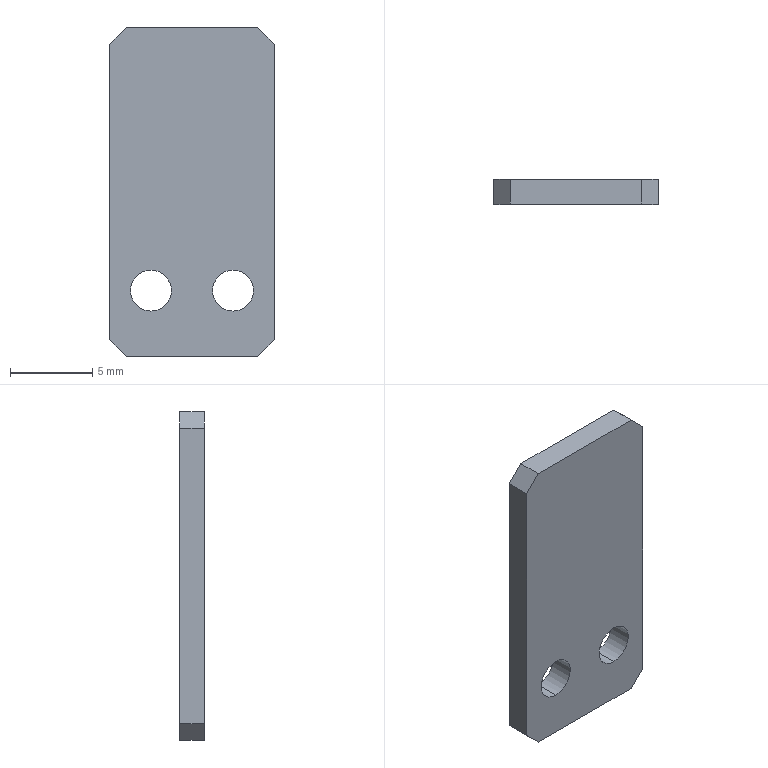Part | SolidWorks | features 3DProfileFeature 1, Chamfer 1, Extrusion 1, HoleWzd 1 | 1 solid | 14 faces | box 10 x 1.5 x 20 mm | volume 282.274 mm3 | plane 10 | cylinder 4 | commonest cylinder face diameters 2.5 x4
STEP:
#1=CARTESIAN_POINT('',(-2.5,0.,-7.25));
#2=VERTEX_POINT('',#1);
#3=CARTESIAN_POINT('',(-2.5,0.,-4.75));
#4=VERTEX_POINT('',#3);
#5=CARTESIAN_POINT('',(-2.5,0.,-6.));
#6=DIRECTION('',(0.,1.,0.));
#7=DIRECTION('',(0.,0.,1.));
#8=AXIS2_PLACEMENT_3D('',#5,#6,#7);
#9=CIRCLE('',#8,1.25);
#10=EDGE_CURVE('',#2,#4,#9,.T.);
#11=ORIENTED_EDGE('',*,*,#10,.F.);
#12=CARTESIAN_POINT('',(-2.5,1.5,-7.25));
#13=VERTEX_POINT('',#12);
#14=CARTESIAN_POINT('',(-2.5,1.5,-7.25));
#15=DIRECTION('',(0.,1.,0.));
#16=VECTOR('',#15,1000.);
#17=LINE('',#14,#16);
#18=EDGE_CURVE('',#2,#13,#17,.T.);
#19=ORIENTED_EDGE('',*,*,#18,.T.);
#20=CARTESIAN_POINT('',(-2.5,1.5,-4.75));
#21=VERTEX_POINT('',#20);
#22=CARTESIAN_POINT('',(-2.5,1.5,-6.));
#23=DIRECTION('',(0.,1.,0.));
#24=DIRECTION('',(0.,0.,1.));
#25=AXIS2_PLACEMENT_3D('',#22,#23,#24);
#26=CIRCLE('',#25,1.25);
#27=EDGE_CURVE('',#13,#21,#26,.T.);
#28=ORIENTED_EDGE('',*,*,#27,.T.);
#29=CARTESIAN_POINT('',(-2.5,1.5,-4.75));
#30=DIRECTION('',(0.,1.,0.));
#31=VECTOR('',#30,1000.);
#32=LINE('',#29,#31);
#33=EDGE_CURVE('',#4,#21,#32,.T.);
#34=ORIENTED_EDGE('',*,*,#33,.F.);
#35=EDGE_LOOP('',(#11,#19,#28,#34));
#36=FACE_OUTER_BOUND('',#35,.T.);
#37=CARTESIAN_POINT('',(-2.5,1.5,-6.));
#38=DIRECTION('',(0.,1.,0.));
#39=DIRECTION('',(0.,0.,1.));
#40=AXIS2_PLACEMENT_3D('',#37,#38,#39);
#41=CYLINDRICAL_SURFACE('',#40,1.25);
#42=ADVANCED_FACE('',(#36),#41,.F.);
#43=CARTESIAN_POINT('',(2.5,0.,-7.25));
#44=VERTEX_POINT('',#43);
#45=CARTESIAN_POINT('',(2.5,0.,-4.75));
#46=VERTEX_POINT('',#45);
#47=CARTESIAN_POINT('',(2.5,0.,-6.));
#48=DIRECTION('',(0.,1.,0.));
#49=DIRECTION('',(0.,0.,1.));
#50=AXIS2_PLACEMENT_3D('',#47,#48,#49);
#51=CIRCLE('',#50,1.25);
#52=EDGE_CURVE('',#44,#46,#51,.T.);
#53=ORIENTED_EDGE('',*,*,#52,.F.);
#54=CARTESIAN_POINT('',(2.5,1.5,-7.25));
#55=VERTEX_POINT('',#54);
#56=CARTESIAN_POINT('',(2.5,1.5,-7.25));
#57=DIRECTION('',(0.,1.,0.));
#58=VECTOR('',#57,1000.);
#59=LINE('',#56,#58);
#60=EDGE_CURVE('',#44,#55,#59,.T.);
#61=ORIENTED_EDGE('',*,*,#60,.T.);
#62=CARTESIAN_POINT('',(2.5,1.5,-4.75));
#63=VERTEX_POINT('',#62);
#64=CARTESIAN_POINT('',(2.5,1.5,-6.));
#65=DIRECTION('',(0.,1.,0.));
#66=DIRECTION('',(0.,0.,1.));
#67=AXIS2_PLACEMENT_3D('',#64,#65,#66);
#68=CIRCLE('',#67,1.25);
#69=EDGE_CURVE('',#55,#63,#68,.T.);
#70=ORIENTED_EDGE('',*,*,#69,.T.);
#71=CARTESIAN_POINT('',(2.5,1.5,-4.75));
#72=DIRECTION('',(0.,1.,0.));
#73=VECTOR('',#72,1000.);
#74=LINE('',#71,#73);
#75=EDGE_CURVE('',#46,#63,#74,.T.);
#76=ORIENTED_EDGE('',*,*,#75,.F.);
#77=EDGE_LOOP('',(#53,#61,#70,#76));
#78=FACE_OUTER_BOUND('',#77,.T.);
#79=CARTESIAN_POINT('',(2.5,1.5,-6.));
#80=DIRECTION('',(0.,1.,0.));
#81=DIRECTION('',(0.,0.,1.));
#82=AXIS2_PLACEMENT_3D('',#79,#80,#81);
#83=CYLINDRICAL_SURFACE('',#82,1.25);
#84=ADVANCED_FACE('',(#78),#83,.F.);
#85=CARTESIAN_POINT('',(5.,1.5,9.));
#86=VERTEX_POINT('',#85);
#87=CARTESIAN_POINT('',(5.,1.5,-9.));
#88=VERTEX_POINT('',#87);
#89=CARTESIAN_POINT('',(5.,1.5,-10.));
#90=DIRECTION('',(0.,0.,-1.));
#91=VECTOR('',#90,1000.);
#92=LINE('',#89,#91);
#93=EDGE_CURVE('',#86,#88,#92,.T.);
#94=ORIENTED_EDGE('',*,*,#93,.F.);
#95=CARTESIAN_POINT('',(5.,0.,9.));
#96=VERTEX_POINT('',#95);
#97=CARTESIAN_POINT('',(5.,1.5,9.));
#98=DIRECTION('',(0.,-1.,0.));
#99=VECTOR('',#98,1000.);
#100=LINE('',#97,#99);
#101=EDGE_CURVE('',#86,#96,#100,.T.);
#102=ORIENTED_EDGE('',*,*,#101,.T.);
#103=CARTESIAN_POINT('',(5.,0.,-9.));
#104=VERTEX_POINT('',#103);
#105=CARTESIAN_POINT('',(5.,0.,-10.));
#106=DIRECTION('',(0.,0.,-1.));
#107=VECTOR('',#106,1000.);
#108=LINE('',#105,#107);
#109=EDGE_CURVE('',#96,#104,#108,.T.);
#110=ORIENTED_EDGE('',*,*,#109,.T.);
#111=CARTESIAN_POINT('',(5.,1.5,-9.));
#112=DIRECTION('',(0.,1.,0.));
#113=VECTOR('',#112,1000.);
#114=LINE('',#111,#113);
#115=EDGE_CURVE('',#104,#88,#114,.T.);
#116=ORIENTED_EDGE('',*,*,#115,.T.);
#117=EDGE_LOOP('',(#94,#102,#110,#116));
#118=FACE_OUTER_BOUND('',#117,.T.);
#119=CARTESIAN_POINT('',(5.,1.5,-10.));
#120=DIRECTION('',(-1.,0.,0.));
#121=DIRECTION('',(0.,0.,1.));
#122=AXIS2_PLACEMENT_3D('',#119,#120,#121);
#123=PLANE('',#122);
#124=ADVANCED_FACE('',(#118),#123,.F.);
#125=CARTESIAN_POINT('',(4.,1.5,-10.));
#126=VERTEX_POINT('',#125);
#127=CARTESIAN_POINT('',(-4.,1.5,-10.));
#128=VERTEX_POINT('',#127);
#129=CARTESIAN_POINT('',(-5.,1.5,-10.));
#130=DIRECTION('',(-1.,0.,0.));
#131=VECTOR('',#130,1000.);
#132=LINE('',#129,#131);
#133=EDGE_CURVE('',#126,#128,#132,.T.);
#134=ORIENTED_EDGE('',*,*,#133,.F.);
#135=CARTESIAN_POINT('',(4.,0.,-10.));
#136=VERTEX_POINT('',#135);
#137=CARTESIAN_POINT('',(4.,1.5,-10.));
#138=DIRECTION('',(0.,-1.,0.));
#139=VECTOR('',#138,1000.);
#140=LINE('',#137,#139);
#141=EDGE_CURVE('',#126,#136,#140,.T.);
#142=ORIENTED_EDGE('',*,*,#141,.T.);
#143=CARTESIAN_POINT('',(-4.,0.,-10.));
#144=VERTEX_POINT('',#143);
#145=CARTESIAN_POINT('',(-5.,0.,-10.));
#146=DIRECTION('',(-1.,0.,0.));
#147=VECTOR('',#146,1000.);
#148=LINE('',#145,#147);
#149=EDGE_CURVE('',#136,#144,#148,.T.);
#150=ORIENTED_EDGE('',*,*,#149,.T.);
#151=CARTESIAN_POINT('',(-4.,1.5,-10.));
#152=DIRECTION('',(0.,1.,0.));
#153=VECTOR('',#152,1000.);
#154=LINE('',#151,#153);
#155=EDGE_CURVE('',#144,#128,#154,.T.);
#156=ORIENTED_EDGE('',*,*,#155,.T.);
#157=EDGE_LOOP('',(#134,#142,#150,#156));
#158=FACE_OUTER_BOUND('',#157,.T.);
#159=CARTESIAN_POINT('',(-5.,1.5,-10.));
#160=DIRECTION('',(0.,0.,1.));
#161=DIRECTION('',(1.,0.,0.));
#162=AXIS2_PLACEMENT_3D('',#159,#160,#161);
#163=PLANE('',#162);
#164=ADVANCED_FACE('',(#158),#163,.F.);
#165=CARTESIAN_POINT('',(-5.,0.,-9.));
#166=VERTEX_POINT('',#165);
#167=CARTESIAN_POINT('',(-5.,0.,9.));
#168=VERTEX_POINT('',#167);
#169=CARTESIAN_POINT('',(-5.,0.,-10.));
#170=DIRECTION('',(0.,0.,1.));
#171=VECTOR('',#170,1000.);
#172=LINE('',#169,#171);
#173=EDGE_CURVE('',#166,#168,#172,.T.);
#174=ORIENTED_EDGE('',*,*,#173,.T.);
#175=CARTESIAN_POINT('',(-5.,1.5,9.));
#176=VERTEX_POINT('',#175);
#177=CARTESIAN_POINT('',(-5.,1.5,9.));
#178=DIRECTION('',(0.,1.,0.));
#179=VECTOR('',#178,1000.);
#180=LINE('',#177,#179);
#181=EDGE_CURVE('',#168,#176,#180,.T.);
#182=ORIENTED_EDGE('',*,*,#181,.T.);
#183=CARTESIAN_POINT('',(-5.,1.5,-9.));
#184=VERTEX_POINT('',#183);
#185=CARTESIAN_POINT('',(-5.,1.5,-10.));
#186=DIRECTION('',(0.,0.,1.));
#187=VECTOR('',#186,1000.);
#188=LINE('',#185,#187);
#189=EDGE_CURVE('',#184,#176,#188,.T.);
#190=ORIENTED_EDGE('',*,*,#189,.F.);
#191=CARTESIAN_POINT('',(-5.,1.5,-9.));
#192=DIRECTION('',(0.,-1.,0.));
#193=VECTOR('',#192,1000.);
#194=LINE('',#191,#193);
#195=EDGE_CURVE('',#184,#166,#194,.T.);
#196=ORIENTED_EDGE('',*,*,#195,.T.);
#197=EDGE_LOOP('',(#174,#182,#190,#196));
#198=FACE_OUTER_BOUND('',#197,.T.);
#199=CARTESIAN_POINT('',(-5.,1.5,-10.));
#200=DIRECTION('',(1.,0.,0.));
#201=DIRECTION('',(0.,0.,-1.));
#202=AXIS2_PLACEMENT_3D('',#199,#200,#201);
#203=PLANE('',#202);
#204=ADVANCED_FACE('',(#198),#203,.F.);
#205=CARTESIAN_POINT('',(-4.,1.5,10.));
#206=VERTEX_POINT('',#205);
#207=CARTESIAN_POINT('',(4.,1.5,10.));
#208=VERTEX_POINT('',#207);
#209=CARTESIAN_POINT('',(-5.,1.5,10.));
#210=DIRECTION('',(1.,0.,0.));
#211=VECTOR('',#210,1000.);
#212=LINE('',#209,#211);
#213=EDGE_CURVE('',#206,#208,#212,.T.);
#214=ORIENTED_EDGE('',*,*,#213,.F.);
#215=CARTESIAN_POINT('',(-4.,0.,10.));
#216=VERTEX_POINT('',#215);
#217=CARTESIAN_POINT('',(-4.,1.5,10.));
#218=DIRECTION('',(0.,-1.,0.));
#219=VECTOR('',#218,1000.);
#220=LINE('',#217,#219);
#221=EDGE_CURVE('',#206,#216,#220,.T.);
#222=ORIENTED_EDGE('',*,*,#221,.T.);
#223=CARTESIAN_POINT('',(4.,0.,10.));
#224=VERTEX_POINT('',#223);
#225=CARTESIAN_POINT('',(-5.,0.,10.));
#226=DIRECTION('',(1.,0.,0.));
#227=VECTOR('',#226,1000.);
#228=LINE('',#225,#227);
#229=EDGE_CURVE('',#216,#224,#228,.T.);
#230=ORIENTED_EDGE('',*,*,#229,.T.);
#231=CARTESIAN_POINT('',(4.,1.5,10.));
#232=DIRECTION('',(0.,1.,0.));
#233=VECTOR('',#232,1000.);
#234=LINE('',#231,#233);
#235=EDGE_CURVE('',#224,#208,#234,.T.);
#236=ORIENTED_EDGE('',*,*,#235,.T.);
#237=EDGE_LOOP('',(#214,#222,#230,#236));
#238=FACE_OUTER_BOUND('',#237,.T.);
#239=CARTESIAN_POINT('',(-5.,1.5,10.));
#240=DIRECTION('',(0.,0.,-1.));
#241=DIRECTION('',(-1.,0.,0.));
#242=AXIS2_PLACEMENT_3D('',#239,#240,#241);
#243=PLANE('',#242);
#244=ADVANCED_FACE('',(#238),#243,.F.);
#245=CARTESIAN_POINT('',(-2.5,1.5,-6.));
#246=DIRECTION('',(0.,1.,0.));
#247=DIRECTION('',(0.,0.,1.));
#248=AXIS2_PLACEMENT_3D('',#245,#246,#247);
#249=CIRCLE('',#248,1.25);
#250=EDGE_CURVE('',#21,#13,#249,.T.);
#251=ORIENTED_EDGE('',*,*,#250,.F.);
#252=ORIENTED_EDGE('',*,*,#27,.F.);
#253=EDGE_LOOP('',(#251,#252));
#254=FACE_BOUND('',#253,.T.);
#255=CARTESIAN_POINT('',(2.5,1.5,-6.));
#256=DIRECTION('',(0.,1.,0.));
#257=DIRECTION('',(0.,0.,1.));
#258=AXIS2_PLACEMENT_3D('',#255,#256,#257);
#259=CIRCLE('',#258,1.25);
#260=EDGE_CURVE('',#63,#55,#259,.T.);
#261=ORIENTED_EDGE('',*,*,#260,.F.);
#262=ORIENTED_EDGE('',*,*,#69,.F.);
#263=EDGE_LOOP('',(#261,#262));
#264=FACE_BOUND('',#263,.T.);
#265=ORIENTED_EDGE('',*,*,#189,.T.);
#266=CARTESIAN_POINT('',(-7.,1.5,7.));
#267=DIRECTION('',(0.7071,0.,0.7071));
#268=VECTOR('',#267,1000.);
#269=LINE('',#266,#268);
#270=EDGE_CURVE('',#176,#206,#269,.T.);
#271=ORIENTED_EDGE('',*,*,#270,.T.);
#272=ORIENTED_EDGE('',*,*,#213,.T.);
#273=CARTESIAN_POINT('',(7.,1.5,7.));
#274=DIRECTION('',(0.7071,0.,-0.7071));
#275=VECTOR('',#274,1000.);
#276=LINE('',#273,#275);
#277=EDGE_CURVE('',#208,#86,#276,.T.);
#278=ORIENTED_EDGE('',*,*,#277,.T.);
#279=ORIENTED_EDGE('',*,*,#93,.T.);
#280=CARTESIAN_POINT('',(7.,1.5,-7.));
#281=DIRECTION('',(-0.7071,0.,-0.7071));
#282=VECTOR('',#281,1000.);
#283=LINE('',#280,#282);
#284=EDGE_CURVE('',#88,#126,#283,.T.);
#285=ORIENTED_EDGE('',*,*,#284,.T.);
#286=ORIENTED_EDGE('',*,*,#133,.T.);
#287=CARTESIAN_POINT('',(-7.,1.5,-7.));
#288=DIRECTION('',(-0.7071,0.,0.7071));
#289=VECTOR('',#288,1000.);
#290=LINE('',#287,#289);
#291=EDGE_CURVE('',#128,#184,#290,.T.);
#292=ORIENTED_EDGE('',*,*,#291,.T.);
#293=EDGE_LOOP('',(#265,#271,#272,#278,#279,#285,#286,#292));
#294=FACE_OUTER_BOUND('',#293,.T.);
#295=CARTESIAN_POINT('',(0.,1.5,0.));
#296=DIRECTION('',(0.,1.,0.));
#297=DIRECTION('',(0.,0.,1.));
#298=AXIS2_PLACEMENT_3D('',#295,#296,#297);
#299=PLANE('',#298);
#300=ADVANCED_FACE('',(#254,#264,#294),#299,.T.);
#301=CARTESIAN_POINT('',(-2.5,0.,-6.));
#302=DIRECTION('',(0.,1.,0.));
#303=DIRECTION('',(0.,0.,1.));
#304=AXIS2_PLACEMENT_3D('',#301,#302,#303);
#305=CIRCLE('',#304,1.25);
#306=EDGE_CURVE('',#4,#2,#305,.T.);
#307=ORIENTED_EDGE('',*,*,#306,.T.);
#308=ORIENTED_EDGE('',*,*,#10,.T.);
#309=EDGE_LOOP('',(#307,#308));
#310=FACE_BOUND('',#309,.T.);
#311=CARTESIAN_POINT('',(2.5,0.,-6.));
#312=DIRECTION('',(0.,1.,0.));
#313=DIRECTION('',(0.,0.,1.));
#314=AXIS2_PLACEMENT_3D('',#311,#312,#313);
#315=CIRCLE('',#314,1.25);
#316=EDGE_CURVE('',#46,#44,#315,.T.);
#317=ORIENTED_EDGE('',*,*,#316,.T.);
#318=ORIENTED_EDGE('',*,*,#52,.T.);
#319=EDGE_LOOP('',(#317,#318));
#320=FACE_BOUND('',#319,.T.);
#321=ORIENTED_EDGE('',*,*,#229,.F.);
#322=CARTESIAN_POINT('',(-4.,0.,10.));
#323=DIRECTION('',(-0.7071,0.,-0.7071));
#324=VECTOR('',#323,1000.);
#325=LINE('',#322,#324);
#326=EDGE_CURVE('',#216,#168,#325,.T.);
#327=ORIENTED_EDGE('',*,*,#326,.T.);
#328=ORIENTED_EDGE('',*,*,#173,.F.);
#329=CARTESIAN_POINT('',(-5.,0.,-9.));
#330=DIRECTION('',(0.7071,0.,-0.7071));
#331=VECTOR('',#330,1000.);
#332=LINE('',#329,#331);
#333=EDGE_CURVE('',#166,#144,#332,.T.);
#334=ORIENTED_EDGE('',*,*,#333,.T.);
#335=ORIENTED_EDGE('',*,*,#149,.F.);
#336=CARTESIAN_POINT('',(4.,0.,-10.));
#337=DIRECTION('',(0.7071,0.,0.7071));
#338=VECTOR('',#337,1000.);
#339=LINE('',#336,#338);
#340=EDGE_CURVE('',#136,#104,#339,.T.);
#341=ORIENTED_EDGE('',*,*,#340,.T.);
#342=ORIENTED_EDGE('',*,*,#109,.F.);
#343=CARTESIAN_POINT('',(5.,0.,9.));
#344=DIRECTION('',(-0.7071,0.,0.7071));
#345=VECTOR('',#344,1000.);
#346=LINE('',#343,#345);
#347=EDGE_CURVE('',#96,#224,#346,.T.);
#348=ORIENTED_EDGE('',*,*,#347,.T.);
#349=EDGE_LOOP('',(#321,#327,#328,#334,#335,#341,#342,#348));
#350=FACE_OUTER_BOUND('',#349,.T.);
#351=CARTESIAN_POINT('',(0.,0.,0.));
#352=DIRECTION('',(0.,1.,0.));
#353=DIRECTION('',(0.,0.,1.));
#354=AXIS2_PLACEMENT_3D('',#351,#352,#353);
#355=PLANE('',#354);
#356=ADVANCED_FACE('',(#310,#320,#350),#355,.F.);
#357=ORIENTED_EDGE('',*,*,#270,.F.);
#358=ORIENTED_EDGE('',*,*,#181,.F.);
#359=ORIENTED_EDGE('',*,*,#326,.F.);
#360=ORIENTED_EDGE('',*,*,#221,.F.);
#361=EDGE_LOOP('',(#357,#358,#359,#360));
#362=FACE_OUTER_BOUND('',#361,.T.);
#363=CARTESIAN_POINT('',(-4.,1.5,10.));
#364=DIRECTION('',(0.7071,0.,-0.7071));
#365=DIRECTION('',(0.,-1.,0.));
#366=AXIS2_PLACEMENT_3D('',#363,#364,#365);
#367=PLANE('',#366);
#368=ADVANCED_FACE('',(#362),#367,.F.);
#369=ORIENTED_EDGE('',*,*,#277,.F.);
#370=ORIENTED_EDGE('',*,*,#235,.F.);
#371=ORIENTED_EDGE('',*,*,#347,.F.);
#372=ORIENTED_EDGE('',*,*,#101,.F.);
#373=EDGE_LOOP('',(#369,#370,#371,#372));
#374=FACE_OUTER_BOUND('',#373,.T.);
#375=CARTESIAN_POINT('',(5.,1.5,9.));
#376=DIRECTION('',(-0.7071,0.,-0.7071));
#377=DIRECTION('',(0.,-1.,0.));
#378=AXIS2_PLACEMENT_3D('',#375,#376,#377);
#379=PLANE('',#378);
#380=ADVANCED_FACE('',(#374),#379,.F.);
#381=ORIENTED_EDGE('',*,*,#284,.F.);
#382=ORIENTED_EDGE('',*,*,#115,.F.);
#383=ORIENTED_EDGE('',*,*,#340,.F.);
#384=ORIENTED_EDGE('',*,*,#141,.F.);
#385=EDGE_LOOP('',(#381,#382,#383,#384));
#386=FACE_OUTER_BOUND('',#385,.T.);
#387=CARTESIAN_POINT('',(4.,1.5,-10.));
#388=DIRECTION('',(-0.7071,0.,0.7071));
#389=DIRECTION('',(0.,-1.,0.));
#390=AXIS2_PLACEMENT_3D('',#387,#388,#389);
#391=PLANE('',#390);
#392=ADVANCED_FACE('',(#386),#391,.F.);
#393=ORIENTED_EDGE('',*,*,#291,.F.);
#394=ORIENTED_EDGE('',*,*,#155,.F.);
#395=ORIENTED_EDGE('',*,*,#333,.F.);
#396=ORIENTED_EDGE('',*,*,#195,.F.);
#397=EDGE_LOOP('',(#393,#394,#395,#396));
#398=FACE_OUTER_BOUND('',#397,.T.);
#399=CARTESIAN_POINT('',(-5.,1.5,-9.));
#400=DIRECTION('',(0.7071,0.,0.7071));
#401=DIRECTION('',(0.,-1.,0.));
#402=AXIS2_PLACEMENT_3D('',#399,#400,#401);
#403=PLANE('',#402);
#404=ADVANCED_FACE('',(#398),#403,.F.);
#405=ORIENTED_EDGE('',*,*,#60,.F.);
#406=ORIENTED_EDGE('',*,*,#316,.F.);
#407=ORIENTED_EDGE('',*,*,#75,.T.);
#408=ORIENTED_EDGE('',*,*,#260,.T.);
#409=EDGE_LOOP('',(#405,#406,#407,#408));
#410=FACE_OUTER_BOUND('',#409,.T.);
#411=CARTESIAN_POINT('',(2.5,1.5,-6.));
#412=DIRECTION('',(0.,1.,0.));
#413=DIRECTION('',(0.,0.,1.));
#414=AXIS2_PLACEMENT_3D('',#411,#412,#413);
#415=CYLINDRICAL_SURFACE('',#414,1.25);
#416=ADVANCED_FACE('',(#410),#415,.F.);
#417=ORIENTED_EDGE('',*,*,#18,.F.);
#418=ORIENTED_EDGE('',*,*,#306,.F.);
#419=ORIENTED_EDGE('',*,*,#33,.T.);
#420=ORIENTED_EDGE('',*,*,#250,.T.);
#421=EDGE_LOOP('',(#417,#418,#419,#420));
#422=FACE_OUTER_BOUND('',#421,.T.);
#423=CARTESIAN_POINT('',(-2.5,1.5,-6.));
#424=DIRECTION('',(0.,1.,0.));
#425=DIRECTION('',(0.,0.,1.));
#426=AXIS2_PLACEMENT_3D('',#423,#424,#425);
#427=CYLINDRICAL_SURFACE('',#426,1.25);
#428=ADVANCED_FACE('',(#422),#427,.F.);
#429=CLOSED_SHELL('',(#42,#84,#124,#164,#204,#244,#300,#356,#368,#380,#392,#404,#416,#428));
#430=MANIFOLD_SOLID_BREP('',#429);
#431=CARTESIAN_POINT('',(0.,0.,0.));
#432=DIRECTION('',(0.,0.,1.));
#433=DIRECTION('',(1.,0.,0.));
#434=AXIS2_PLACEMENT_3D('',#431,#432,#433);
#435=(LENGTH_UNIT()NAMED_UNIT(*)SI_UNIT(.MILLI.,.METRE.));
#436=UNCERTAINTY_MEASURE_WITH_UNIT(LENGTH_MEASURE(0.00001),#435,'','');
#437=(NAMED_UNIT(*)PLANE_ANGLE_UNIT()SI_UNIT($,.RADIAN.));
#438=(NAMED_UNIT(*)SI_UNIT($,.STERADIAN.)SOLID_ANGLE_UNIT());
#439=(GEOMETRIC_REPRESENTATION_CONTEXT(3)GLOBAL_UNCERTAINTY_ASSIGNED_CONTEXT((#436))GLOBAL_UNIT_ASSIGNED_CONTEXT((#435,#437,#438))REPRESENTATION_CONTEXT('',''));
#440=ADVANCED_BREP_SHAPE_REPRESENTATION('',(#430,#434),#439);